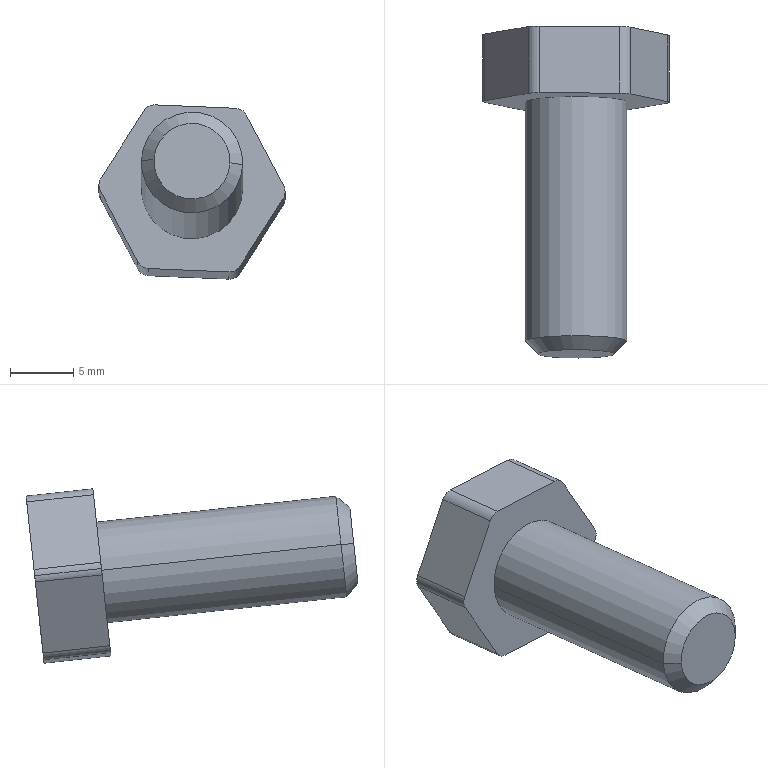Part | STEP file | Chamfer 2-4 | 1 solid | 21 faces | box 14.69 x 26.187 x 13.75 mm | volume 1768 mm3 | cylinder 10 | plane 9 | cone 2 | commonest cylinder face diameters 2 x8 8 x2
STEP:
#1=CARTESIAN_POINT('',(298.084,-1236.553,3544.637));
#2=VERTEX_POINT('',#1);
#3=CARTESIAN_POINT('',(297.929,-1236.606,3544.146));
#4=VERTEX_POINT('',#3);
#5=CARTESIAN_POINT('',(297.085,-1236.548,3544.679));
#6=DIRECTION('',(0.,0.9942,-0.1073));
#7=DIRECTION('',(0.9991,-0.004526,-0.04193));
#8=AXIS2_PLACEMENT_3D('',#5,#6,#7);
#9=CIRCLE('',#8,1.);
#10=EDGE_CURVE('',#2,#4,#9,.T.);
#11=ORIENTED_EDGE('',*,*,#10,.F.);
#12=CARTESIAN_POINT('',(298.084,-1241.822,3545.206));
#13=VERTEX_POINT('',#12);
#14=CARTESIAN_POINT('',(298.084,-1236.553,3544.637));
#15=DIRECTION('',(0.,-0.9942,0.1073));
#16=VECTOR('',#15,1000.);
#17=LINE('',#14,#16);
#18=EDGE_CURVE('',#2,#13,#17,.T.);
#19=ORIENTED_EDGE('',*,*,#18,.T.);
#20=CARTESIAN_POINT('',(297.929,-1241.875,3544.715));
#21=VERTEX_POINT('',#20);
#22=CARTESIAN_POINT('',(297.085,-1241.818,3545.248));
#23=DIRECTION('',(0.,-0.9942,0.1073));
#24=DIRECTION('',(0.9991,-0.004526,-0.04193));
#25=AXIS2_PLACEMENT_3D('',#22,#23,#24);
#26=CIRCLE('',#25,1.);
#27=EDGE_CURVE('',#21,#13,#26,.T.);
#28=ORIENTED_EDGE('',*,*,#27,.F.);
#29=CARTESIAN_POINT('',(297.929,-1236.606,3544.146));
#30=DIRECTION('',(0.,-0.9942,0.1073));
#31=VECTOR('',#30,1000.);
#32=LINE('',#29,#31);
#33=EDGE_CURVE('',#4,#21,#32,.T.);
#34=ORIENTED_EDGE('',*,*,#33,.F.);
#35=EDGE_LOOP('',(#11,#19,#28,#34));
#36=FACE_OUTER_BOUND('',#35,.T.);
#37=CARTESIAN_POINT('',(297.085,-1236.548,3544.679));
#38=DIRECTION('',(0.,-0.9942,0.1073));
#39=DIRECTION('',(0.9991,-0.004526,-0.04193));
#40=AXIS2_PLACEMENT_3D('',#37,#38,#39);
#41=CYLINDRICAL_SURFACE('',#40,1.);
#42=ADVANCED_FACE('',(#36),#41,.T.);
#43=CARTESIAN_POINT('',(287.742,-1261.66,3547.787));
#44=VERTEX_POINT('',#43);
#45=CARTESIAN_POINT('',(293.737,-1261.687,3547.536));
#46=VERTEX_POINT('',#45);
#47=CARTESIAN_POINT('',(290.74,-1261.674,3547.661));
#48=DIRECTION('',(0.,-0.9942,0.1073));
#49=DIRECTION('',(0.9991,-0.004526,-0.04193));
#50=AXIS2_PLACEMENT_3D('',#47,#48,#49);
#51=CIRCLE('',#50,3.);
#52=EDGE_CURVE('',#44,#46,#51,.T.);
#53=ORIENTED_EDGE('',*,*,#52,.F.);
#54=CARTESIAN_POINT('',(286.743,-1260.661,3547.722));
#55=VERTEX_POINT('',#54);
#56=CARTESIAN_POINT('',(286.743,-1260.661,3547.722));
#57=DIRECTION('',(-0.7065,0.7062,-0.04626));
#58=VECTOR('',#57,1000.);
#59=LINE('',#56,#58);
#60=EDGE_CURVE('',#44,#55,#59,.T.);
#61=ORIENTED_EDGE('',*,*,#60,.T.);
#62=CARTESIAN_POINT('',(294.736,-1260.697,3547.386));
#63=VERTEX_POINT('',#62);
#64=CARTESIAN_POINT('',(290.74,-1260.679,3547.554));
#65=DIRECTION('',(0.,0.9942,-0.1073));
#66=DIRECTION('',(0.9991,-0.004526,-0.04193));
#67=AXIS2_PLACEMENT_3D('',#64,#65,#66);
#68=CIRCLE('',#67,4.);
#69=EDGE_CURVE('',#63,#55,#68,.T.);
#70=ORIENTED_EDGE('',*,*,#69,.F.);
#71=CARTESIAN_POINT('',(294.736,-1260.697,3547.386));
#72=DIRECTION('',(0.7065,0.6998,-0.1055));
#73=VECTOR('',#72,1000.);
#74=LINE('',#71,#73);
#75=EDGE_CURVE('',#46,#63,#74,.T.);
#76=ORIENTED_EDGE('',*,*,#75,.F.);
#77=EDGE_LOOP('',(#53,#61,#70,#76));
#78=FACE_OUTER_BOUND('',#77,.T.);
#79=CARTESIAN_POINT('',(290.74,-1260.679,3547.554));
#80=DIRECTION('',(0.,0.9942,-0.1073));
#81=DIRECTION('',(-0.9991,0.004526,0.04193));
#82=AXIS2_PLACEMENT_3D('',#79,#80,#81);
#83=CONICAL_SURFACE('',#82,4.,0.7854);
#84=ADVANCED_FACE('',(#78),#83,.T.);
#85=ORIENTED_EDGE('',*,*,#69,.T.);
#86=CARTESIAN_POINT('',(286.743,-1241.771,3545.682));
#87=VERTEX_POINT('',#86);
#88=CARTESIAN_POINT('',(286.743,-1261.655,3547.829));
#89=DIRECTION('',(0.,0.9942,-0.1073));
#90=VECTOR('',#89,1000.);
#91=LINE('',#88,#90);
#92=EDGE_CURVE('',#55,#87,#91,.T.);
#93=ORIENTED_EDGE('',*,*,#92,.T.);
#94=CARTESIAN_POINT('',(294.736,-1241.807,3545.347));
#95=VERTEX_POINT('',#94);
#96=CARTESIAN_POINT('',(290.74,-1241.789,3545.515));
#97=DIRECTION('',(0.,0.9942,-0.1073));
#98=DIRECTION('',(0.9991,-0.004526,-0.04193));
#99=AXIS2_PLACEMENT_3D('',#96,#97,#98);
#100=CIRCLE('',#99,4.);
#101=EDGE_CURVE('',#95,#87,#100,.T.);
#102=ORIENTED_EDGE('',*,*,#101,.F.);
#103=CARTESIAN_POINT('',(294.736,-1261.692,3547.494));
#104=DIRECTION('',(0.,0.9942,-0.1073));
#105=VECTOR('',#104,1000.);
#106=LINE('',#103,#105);
#107=EDGE_CURVE('',#63,#95,#106,.T.);
#108=ORIENTED_EDGE('',*,*,#107,.F.);
#109=EDGE_LOOP('',(#85,#93,#102,#108));
#110=FACE_OUTER_BOUND('',#109,.T.);
#111=CARTESIAN_POINT('',(290.74,-1261.674,3547.661));
#112=DIRECTION('',(0.,0.9942,-0.1073));
#113=DIRECTION('',(-0.9991,0.004526,0.04193));
#114=AXIS2_PLACEMENT_3D('',#111,#112,#113);
#115=CYLINDRICAL_SURFACE('',#114,4.);
#116=ADVANCED_FACE('',(#110),#115,.T.);
#117=CARTESIAN_POINT('',(283.395,-1236.486,3545.254));
#118=VERTEX_POINT('',#117);
#119=CARTESIAN_POINT('',(283.55,-1236.433,3545.745));
#120=VERTEX_POINT('',#119);
#121=CARTESIAN_POINT('',(284.394,-1236.491,3545.212));
#122=DIRECTION('',(0.,0.9942,-0.1073));
#123=DIRECTION('',(0.9991,-0.004526,-0.04193));
#124=AXIS2_PLACEMENT_3D('',#121,#122,#123);
#125=CIRCLE('',#124,1.);
#126=EDGE_CURVE('',#118,#120,#125,.T.);
#127=ORIENTED_EDGE('',*,*,#126,.F.);
#128=CARTESIAN_POINT('',(283.395,-1241.756,3545.823));
#129=VERTEX_POINT('',#128);
#130=CARTESIAN_POINT('',(283.395,-1236.486,3545.254));
#131=DIRECTION('',(0.,-0.9942,0.1073));
#132=VECTOR('',#131,1000.);
#133=LINE('',#130,#132);
#134=EDGE_CURVE('',#118,#129,#133,.T.);
#135=ORIENTED_EDGE('',*,*,#134,.T.);
#136=CARTESIAN_POINT('',(283.55,-1241.703,3546.314));
#137=VERTEX_POINT('',#136);
#138=CARTESIAN_POINT('',(284.394,-1241.76,3545.781));
#139=DIRECTION('',(0.,-0.9942,0.1073));
#140=DIRECTION('',(0.9991,-0.004526,-0.04193));
#141=AXIS2_PLACEMENT_3D('',#138,#139,#140);
#142=CIRCLE('',#141,1.);
#143=EDGE_CURVE('',#137,#129,#142,.T.);
#144=ORIENTED_EDGE('',*,*,#143,.F.);
#145=CARTESIAN_POINT('',(283.55,-1236.433,3545.745));
#146=DIRECTION('',(0.,-0.9942,0.1073));
#147=VECTOR('',#146,1000.);
#148=LINE('',#145,#147);
#149=EDGE_CURVE('',#120,#137,#148,.T.);
#150=ORIENTED_EDGE('',*,*,#149,.F.);
#151=EDGE_LOOP('',(#127,#135,#144,#150));
#152=FACE_OUTER_BOUND('',#151,.T.);
#153=CARTESIAN_POINT('',(284.394,-1236.491,3545.212));
#154=DIRECTION('',(0.,-0.9942,0.1073));
#155=DIRECTION('',(0.9991,-0.004526,-0.04193));
#156=AXIS2_PLACEMENT_3D('',#153,#154,#155);
#157=CYLINDRICAL_SURFACE('',#156,1.);
#158=ADVANCED_FACE('',(#152),#157,.T.);
#159=CARTESIAN_POINT('',(295.03,-1235.895,3550.736));
#160=VERTEX_POINT('',#159);
#161=CARTESIAN_POINT('',(297.971,-1236.499,3545.14));
#162=VERTEX_POINT('',#161);
#163=CARTESIAN_POINT('',(294.763,-1235.84,3551.245));
#164=DIRECTION('',(0.463,-0.09514,-0.8812));
#165=VECTOR('',#164,1000.);
#166=LINE('',#163,#165);
#167=EDGE_CURVE('',#160,#162,#166,.T.);
#168=ORIENTED_EDGE('',*,*,#167,.F.);
#169=CARTESIAN_POINT('',(295.03,-1241.164,3551.305));
#170=VERTEX_POINT('',#169);
#171=CARTESIAN_POINT('',(295.03,-1235.895,3550.736));
#172=DIRECTION('',(0.,-0.9942,0.1073));
#173=VECTOR('',#172,1000.);
#174=LINE('',#171,#173);
#175=EDGE_CURVE('',#160,#170,#174,.T.);
#176=ORIENTED_EDGE('',*,*,#175,.T.);
#177=CARTESIAN_POINT('',(297.971,-1241.768,3545.709));
#178=VERTEX_POINT('',#177);
#179=CARTESIAN_POINT('',(294.763,-1241.109,3551.814));
#180=DIRECTION('',(0.463,-0.09514,-0.8812));
#181=VECTOR('',#180,1000.);
#182=LINE('',#179,#181);
#183=EDGE_CURVE('',#170,#178,#182,.T.);
#184=ORIENTED_EDGE('',*,*,#183,.T.);
#185=CARTESIAN_POINT('',(297.971,-1236.499,3545.14));
#186=DIRECTION('',(0.,0.9942,-0.1073));
#187=VECTOR('',#186,1000.);
#188=LINE('',#185,#187);
#189=EDGE_CURVE('',#178,#162,#188,.T.);
#190=ORIENTED_EDGE('',*,*,#189,.T.);
#191=EDGE_LOOP('',(#168,#176,#184,#190));
#192=FACE_OUTER_BOUND('',#191,.T.);
#193=CARTESIAN_POINT('',(294.763,-1235.84,3551.245));
#194=DIRECTION('',(-0.8863,-0.0497,-0.4604));
#195=DIRECTION('',(0.463,-0.09514,-0.8812));
#196=AXIS2_PLACEMENT_3D('',#193,#194,#195);
#197=PLANE('',#196);
#198=ADVANCED_FACE('',(#192),#197,.F.);
#199=CARTESIAN_POINT('',(294.524,-1242.451,3539.385));
#200=VERTEX_POINT('',#199);
#201=CARTESIAN_POINT('',(298.238,-1241.823,3545.2));
#202=DIRECTION('',(-0.5361,-0.09061,-0.8393));
#203=VECTOR('',#202,1000.);
#204=LINE('',#201,#203);
#205=EDGE_CURVE('',#21,#200,#204,.T.);
#206=ORIENTED_EDGE('',*,*,#205,.T.);
#207=CARTESIAN_POINT('',(294.524,-1237.181,3538.816));
#208=VERTEX_POINT('',#207);
#209=CARTESIAN_POINT('',(294.524,-1237.181,3538.816));
#210=DIRECTION('',(0.,0.9942,-0.1073));
#211=VECTOR('',#210,1000.);
#212=LINE('',#209,#211);
#213=EDGE_CURVE('',#200,#208,#212,.T.);
#214=ORIENTED_EDGE('',*,*,#213,.T.);
#215=CARTESIAN_POINT('',(298.238,-1236.554,3544.631));
#216=DIRECTION('',(-0.5361,-0.09061,-0.8393));
#217=VECTOR('',#216,1000.);
#218=LINE('',#215,#217);
#219=EDGE_CURVE('',#4,#208,#218,.T.);
#220=ORIENTED_EDGE('',*,*,#219,.F.);
#221=ORIENTED_EDGE('',*,*,#33,.T.);
#222=EDGE_LOOP('',(#206,#214,#220,#221));
#223=FACE_OUTER_BOUND('',#222,.T.);
#224=CARTESIAN_POINT('',(298.238,-1236.554,3544.631));
#225=DIRECTION('',(-0.8442,0.05754,0.533));
#226=DIRECTION('',(-0.5361,-0.09061,-0.8393));
#227=AXIS2_PLACEMENT_3D('',#224,#225,#226);
#228=PLANE('',#227);
#229=ADVANCED_FACE('',(#223),#228,.F.);
#230=CARTESIAN_POINT('',(293.638,-1237.231,3538.356));
#231=VERTEX_POINT('',#230);
#232=CARTESIAN_POINT('',(287.293,-1237.202,3538.622));
#233=VERTEX_POINT('',#232);
#234=CARTESIAN_POINT('',(294.215,-1237.234,3538.332));
#235=DIRECTION('',(-0.9991,0.004526,0.04193));
#236=VECTOR('',#235,1000.);
#237=LINE('',#234,#236);
#238=EDGE_CURVE('',#231,#233,#237,.T.);
#239=ORIENTED_EDGE('',*,*,#238,.F.);
#240=CARTESIAN_POINT('',(293.638,-1242.501,3538.925));
#241=VERTEX_POINT('',#240);
#242=CARTESIAN_POINT('',(293.638,-1237.231,3538.356));
#243=DIRECTION('',(0.,-0.9942,0.1073));
#244=VECTOR('',#243,1000.);
#245=LINE('',#242,#244);
#246=EDGE_CURVE('',#231,#241,#245,.T.);
#247=ORIENTED_EDGE('',*,*,#246,.T.);
#248=CARTESIAN_POINT('',(287.293,-1242.472,3539.191));
#249=VERTEX_POINT('',#248);
#250=CARTESIAN_POINT('',(294.215,-1242.503,3538.901));
#251=DIRECTION('',(-0.9991,0.004526,0.04193));
#252=VECTOR('',#251,1000.);
#253=LINE('',#250,#252);
#254=EDGE_CURVE('',#241,#249,#253,.T.);
#255=ORIENTED_EDGE('',*,*,#254,.T.);
#256=CARTESIAN_POINT('',(287.293,-1237.202,3538.622));
#257=DIRECTION('',(0.,0.9942,-0.1073));
#258=VECTOR('',#257,1000.);
#259=LINE('',#256,#258);
#260=EDGE_CURVE('',#249,#233,#259,.T.);
#261=ORIENTED_EDGE('',*,*,#260,.T.);
#262=EDGE_LOOP('',(#239,#247,#255,#261));
#263=FACE_OUTER_BOUND('',#262,.T.);
#264=CARTESIAN_POINT('',(294.215,-1237.234,3538.332));
#265=DIRECTION('',(0.04217,0.1072,0.9933));
#266=DIRECTION('',(0.,0.9942,-0.1073));
#267=AXIS2_PLACEMENT_3D('',#264,#265,#266);
#268=PLANE('',#267);
#269=ADVANCED_FACE('',(#263),#268,.F.);
#270=CARTESIAN_POINT('',(286.449,-1237.145,3539.155));
#271=VERTEX_POINT('',#270);
#272=CARTESIAN_POINT('',(283.508,-1236.541,3544.752));
#273=VERTEX_POINT('',#272);
#274=CARTESIAN_POINT('',(286.716,-1237.2,3538.646));
#275=DIRECTION('',(-0.463,0.09514,0.8812));
#276=VECTOR('',#275,1000.);
#277=LINE('',#274,#276);
#278=EDGE_CURVE('',#271,#273,#277,.T.);
#279=ORIENTED_EDGE('',*,*,#278,.F.);
#280=CARTESIAN_POINT('',(286.449,-1242.414,3539.724));
#281=VERTEX_POINT('',#280);
#282=CARTESIAN_POINT('',(286.449,-1237.145,3539.155));
#283=DIRECTION('',(0.,-0.9942,0.1073));
#284=VECTOR('',#283,1000.);
#285=LINE('',#282,#284);
#286=EDGE_CURVE('',#271,#281,#285,.T.);
#287=ORIENTED_EDGE('',*,*,#286,.T.);
#288=CARTESIAN_POINT('',(283.508,-1241.81,3545.32));
#289=VERTEX_POINT('',#288);
#290=CARTESIAN_POINT('',(286.716,-1242.469,3539.215));
#291=DIRECTION('',(-0.463,0.09514,0.8812));
#292=VECTOR('',#291,1000.);
#293=LINE('',#290,#292);
#294=EDGE_CURVE('',#281,#289,#293,.T.);
#295=ORIENTED_EDGE('',*,*,#294,.T.);
#296=CARTESIAN_POINT('',(283.508,-1236.541,3544.752));
#297=DIRECTION('',(0.,0.9942,-0.1073));
#298=VECTOR('',#297,1000.);
#299=LINE('',#296,#298);
#300=EDGE_CURVE('',#289,#273,#299,.T.);
#301=ORIENTED_EDGE('',*,*,#300,.T.);
#302=EDGE_LOOP('',(#279,#287,#295,#301));
#303=FACE_OUTER_BOUND('',#302,.T.);
#304=CARTESIAN_POINT('',(286.716,-1237.2,3538.646));
#305=DIRECTION('',(0.8863,0.0497,0.4604));
#306=DIRECTION('',(-0.463,0.09514,0.8812));
#307=AXIS2_PLACEMENT_3D('',#304,#305,#306);
#308=PLANE('',#307);
#309=ADVANCED_FACE('',(#303),#308,.F.);
#310=CARTESIAN_POINT('',(286.955,-1235.858,3551.075));
#311=VERTEX_POINT('',#310);
#312=CARTESIAN_POINT('',(283.241,-1236.486,3545.26));
#313=DIRECTION('',(0.5361,0.09061,0.8393));
#314=VECTOR('',#313,1000.);
#315=LINE('',#312,#314);
#316=EDGE_CURVE('',#120,#311,#315,.T.);
#317=ORIENTED_EDGE('',*,*,#316,.F.);
#318=ORIENTED_EDGE('',*,*,#149,.T.);
#319=CARTESIAN_POINT('',(286.955,-1241.127,3551.644));
#320=VERTEX_POINT('',#319);
#321=CARTESIAN_POINT('',(283.241,-1241.755,3545.829));
#322=DIRECTION('',(0.5361,0.09061,0.8393));
#323=VECTOR('',#322,1000.);
#324=LINE('',#321,#323);
#325=EDGE_CURVE('',#137,#320,#324,.T.);
#326=ORIENTED_EDGE('',*,*,#325,.T.);
#327=CARTESIAN_POINT('',(286.955,-1235.858,3551.075));
#328=DIRECTION('',(0.,0.9942,-0.1073));
#329=VECTOR('',#328,1000.);
#330=LINE('',#327,#329);
#331=EDGE_CURVE('',#320,#311,#330,.T.);
#332=ORIENTED_EDGE('',*,*,#331,.T.);
#333=EDGE_LOOP('',(#317,#318,#326,#332));
#334=FACE_OUTER_BOUND('',#333,.T.);
#335=CARTESIAN_POINT('',(283.241,-1236.486,3545.26));
#336=DIRECTION('',(0.8442,-0.05754,-0.533));
#337=DIRECTION('',(0.5361,0.09061,0.8393));
#338=AXIS2_PLACEMENT_3D('',#335,#336,#337);
#339=PLANE('',#338);
#340=ADVANCED_FACE('',(#334),#339,.F.);
#341=CARTESIAN_POINT('',(287.841,-1235.808,3551.535));
#342=VERTEX_POINT('',#341);
#343=CARTESIAN_POINT('',(294.186,-1235.837,3551.269));
#344=VERTEX_POINT('',#343);
#345=CARTESIAN_POINT('',(287.264,-1235.806,3551.56));
#346=DIRECTION('',(0.9991,-0.004526,-0.04193));
#347=VECTOR('',#346,1000.);
#348=LINE('',#345,#347);
#349=EDGE_CURVE('',#342,#344,#348,.T.);
#350=ORIENTED_EDGE('',*,*,#349,.F.);
#351=CARTESIAN_POINT('',(287.841,-1241.078,3552.104));
#352=VERTEX_POINT('',#351);
#353=CARTESIAN_POINT('',(287.841,-1235.808,3551.535));
#354=DIRECTION('',(0.,-0.9942,0.1073));
#355=VECTOR('',#354,1000.);
#356=LINE('',#353,#355);
#357=EDGE_CURVE('',#342,#352,#356,.T.);
#358=ORIENTED_EDGE('',*,*,#357,.T.);
#359=CARTESIAN_POINT('',(294.186,-1241.106,3551.838));
#360=VERTEX_POINT('',#359);
#361=CARTESIAN_POINT('',(287.264,-1241.075,3552.129));
#362=DIRECTION('',(0.9991,-0.004526,-0.04193));
#363=VECTOR('',#362,1000.);
#364=LINE('',#361,#363);
#365=EDGE_CURVE('',#352,#360,#364,.T.);
#366=ORIENTED_EDGE('',*,*,#365,.T.);
#367=CARTESIAN_POINT('',(294.186,-1235.837,3551.269));
#368=DIRECTION('',(0.,0.9942,-0.1073));
#369=VECTOR('',#368,1000.);
#370=LINE('',#367,#369);
#371=EDGE_CURVE('',#360,#344,#370,.T.);
#372=ORIENTED_EDGE('',*,*,#371,.T.);
#373=EDGE_LOOP('',(#350,#358,#366,#372));
#374=FACE_OUTER_BOUND('',#373,.T.);
#375=CARTESIAN_POINT('',(287.264,-1235.806,3551.56));
#376=DIRECTION('',(-0.04217,-0.1072,-0.9933));
#377=DIRECTION('',(0.9991,-0.004526,-0.04193));
#378=AXIS2_PLACEMENT_3D('',#375,#376,#377);
#379=PLANE('',#378);
#380=ADVANCED_FACE('',(#374),#379,.F.);
#381=ORIENTED_EDGE('',*,*,#219,.T.);
#382=CARTESIAN_POINT('',(293.68,-1237.124,3539.349));
#383=DIRECTION('',(0.,0.9942,-0.1073));
#384=DIRECTION('',(0.9991,-0.004526,-0.04193));
#385=AXIS2_PLACEMENT_3D('',#382,#383,#384);
#386=CIRCLE('',#385,1.);
#387=EDGE_CURVE('',#208,#231,#386,.T.);
#388=ORIENTED_EDGE('',*,*,#387,.T.);
#389=ORIENTED_EDGE('',*,*,#238,.T.);
#390=CARTESIAN_POINT('',(287.335,-1237.095,3539.615));
#391=DIRECTION('',(0.,0.9942,-0.1073));
#392=DIRECTION('',(0.9991,-0.004526,-0.04193));
#393=AXIS2_PLACEMENT_3D('',#390,#391,#392);
#394=CIRCLE('',#393,1.);
#395=EDGE_CURVE('',#233,#271,#394,.T.);
#396=ORIENTED_EDGE('',*,*,#395,.T.);
#397=ORIENTED_EDGE('',*,*,#278,.T.);
#398=CARTESIAN_POINT('',(284.394,-1236.491,3545.212));
#399=DIRECTION('',(0.,0.9942,-0.1073));
#400=DIRECTION('',(0.9991,-0.004526,-0.04193));
#401=AXIS2_PLACEMENT_3D('',#398,#399,#400);
#402=CIRCLE('',#401,1.);
#403=EDGE_CURVE('',#273,#118,#402,.T.);
#404=ORIENTED_EDGE('',*,*,#403,.T.);
#405=ORIENTED_EDGE('',*,*,#126,.T.);
#406=ORIENTED_EDGE('',*,*,#316,.T.);
#407=CARTESIAN_POINT('',(287.799,-1235.915,3550.542));
#408=DIRECTION('',(0.,0.9942,-0.1073));
#409=DIRECTION('',(0.9991,-0.004526,-0.04193));
#410=AXIS2_PLACEMENT_3D('',#407,#408,#409);
#411=CIRCLE('',#410,1.);
#412=EDGE_CURVE('',#311,#342,#411,.T.);
#413=ORIENTED_EDGE('',*,*,#412,.T.);
#414=ORIENTED_EDGE('',*,*,#349,.T.);
#415=CARTESIAN_POINT('',(294.144,-1235.944,3550.276));
#416=DIRECTION('',(0.,0.9942,-0.1073));
#417=DIRECTION('',(0.9991,-0.004526,-0.04193));
#418=AXIS2_PLACEMENT_3D('',#415,#416,#417);
#419=CIRCLE('',#418,1.);
#420=EDGE_CURVE('',#344,#160,#419,.T.);
#421=ORIENTED_EDGE('',*,*,#420,.T.);
#422=ORIENTED_EDGE('',*,*,#167,.T.);
#423=CARTESIAN_POINT('',(297.085,-1236.548,3544.679));
#424=DIRECTION('',(0.,0.9942,-0.1073));
#425=DIRECTION('',(0.9991,-0.004526,-0.04193));
#426=AXIS2_PLACEMENT_3D('',#423,#424,#425);
#427=CIRCLE('',#426,1.);
#428=EDGE_CURVE('',#162,#2,#427,.T.);
#429=ORIENTED_EDGE('',*,*,#428,.T.);
#430=ORIENTED_EDGE('',*,*,#10,.T.);
#431=EDGE_LOOP('',(#381,#388,#389,#396,#397,#404,#405,#406,#413,#414,#421,#422,#429,#430));
#432=FACE_OUTER_BOUND('',#431,.T.);
#433=CARTESIAN_POINT('',(293.975,-1236.534,3544.81));
#434=DIRECTION('',(0.,0.9942,-0.1073));
#435=DIRECTION('',(-0.9991,0.004526,0.04193));
#436=AXIS2_PLACEMENT_3D('',#433,#434,#435);
#437=PLANE('',#436);
#438=ADVANCED_FACE('',(#432),#437,.T.);
#439=ORIENTED_EDGE('',*,*,#101,.T.);
#440=CARTESIAN_POINT('',(290.74,-1241.789,3545.515));
#441=DIRECTION('',(0.,0.9942,-0.1073));
#442=DIRECTION('',(0.9991,-0.004526,-0.04193));
#443=AXIS2_PLACEMENT_3D('',#440,#441,#442);
#444=CIRCLE('',#443,4.);
#445=EDGE_CURVE('',#87,#95,#444,.T.);
#446=ORIENTED_EDGE('',*,*,#445,.T.);
#447=EDGE_LOOP('',(#439,#446));
#448=FACE_BOUND('',#447,.T.);
#449=ORIENTED_EDGE('',*,*,#254,.F.);
#450=CARTESIAN_POINT('',(293.68,-1242.393,3539.918));
#451=DIRECTION('',(0.,-0.9942,0.1073));
#452=DIRECTION('',(0.9991,-0.004526,-0.04193));
#453=AXIS2_PLACEMENT_3D('',#450,#451,#452);
#454=CIRCLE('',#453,1.);
#455=EDGE_CURVE('',#241,#200,#454,.T.);
#456=ORIENTED_EDGE('',*,*,#455,.T.);
#457=ORIENTED_EDGE('',*,*,#205,.F.);
#458=ORIENTED_EDGE('',*,*,#27,.T.);
#459=CARTESIAN_POINT('',(297.085,-1241.818,3545.248));
#460=DIRECTION('',(0.,-0.9942,0.1073));
#461=DIRECTION('',(0.9991,-0.004526,-0.04193));
#462=AXIS2_PLACEMENT_3D('',#459,#460,#461);
#463=CIRCLE('',#462,1.);
#464=EDGE_CURVE('',#13,#178,#463,.T.);
#465=ORIENTED_EDGE('',*,*,#464,.T.);
#466=ORIENTED_EDGE('',*,*,#183,.F.);
#467=CARTESIAN_POINT('',(294.144,-1241.214,3550.845));
#468=DIRECTION('',(0.,-0.9942,0.1073));
#469=DIRECTION('',(0.9991,-0.004526,-0.04193));
#470=AXIS2_PLACEMENT_3D('',#467,#468,#469);
#471=CIRCLE('',#470,1.);
#472=EDGE_CURVE('',#170,#360,#471,.T.);
#473=ORIENTED_EDGE('',*,*,#472,.T.);
#474=ORIENTED_EDGE('',*,*,#365,.F.);
#475=CARTESIAN_POINT('',(287.799,-1241.185,3551.111));
#476=DIRECTION('',(0.,-0.9942,0.1073));
#477=DIRECTION('',(0.9991,-0.004526,-0.04193));
#478=AXIS2_PLACEMENT_3D('',#475,#476,#477);
#479=CIRCLE('',#478,1.);
#480=EDGE_CURVE('',#352,#320,#479,.T.);
#481=ORIENTED_EDGE('',*,*,#480,.T.);
#482=ORIENTED_EDGE('',*,*,#325,.F.);
#483=ORIENTED_EDGE('',*,*,#143,.T.);
#484=CARTESIAN_POINT('',(284.394,-1241.76,3545.781));
#485=DIRECTION('',(0.,-0.9942,0.1073));
#486=DIRECTION('',(0.9991,-0.004526,-0.04193));
#487=AXIS2_PLACEMENT_3D('',#484,#485,#486);
#488=CIRCLE('',#487,1.);
#489=EDGE_CURVE('',#129,#289,#488,.T.);
#490=ORIENTED_EDGE('',*,*,#489,.T.);
#491=ORIENTED_EDGE('',*,*,#294,.F.);
#492=CARTESIAN_POINT('',(287.335,-1242.365,3540.184));
#493=DIRECTION('',(0.,-0.9942,0.1073));
#494=DIRECTION('',(0.9991,-0.004526,-0.04193));
#495=AXIS2_PLACEMENT_3D('',#492,#493,#494);
#496=CIRCLE('',#495,1.);
#497=EDGE_CURVE('',#281,#249,#496,.T.);
#498=ORIENTED_EDGE('',*,*,#497,.T.);
#499=EDGE_LOOP('',(#449,#456,#457,#458,#465,#466,#473,#474,#481,#482,#483,#490,#491,#498));
#500=FACE_OUTER_BOUND('',#499,.T.);
#501=CARTESIAN_POINT('',(293.975,-1241.804,3545.379));
#502=DIRECTION('',(0.,0.9942,-0.1073));
#503=DIRECTION('',(-0.9991,0.004526,0.04193));
#504=AXIS2_PLACEMENT_3D('',#501,#502,#503);
#505=PLANE('',#504);
#506=ADVANCED_FACE('',(#448,#500),#505,.F.);
#507=ORIENTED_EDGE('',*,*,#387,.F.);
#508=ORIENTED_EDGE('',*,*,#213,.F.);
#509=ORIENTED_EDGE('',*,*,#455,.F.);
#510=ORIENTED_EDGE('',*,*,#246,.F.);
#511=EDGE_LOOP('',(#507,#508,#509,#510));
#512=FACE_OUTER_BOUND('',#511,.T.);
#513=CARTESIAN_POINT('',(293.68,-1237.124,3539.349));
#514=DIRECTION('',(0.,-0.9942,0.1073));
#515=DIRECTION('',(0.9991,-0.004526,-0.04193));
#516=AXIS2_PLACEMENT_3D('',#513,#514,#515);
#517=CYLINDRICAL_SURFACE('',#516,1.);
#518=ADVANCED_FACE('',(#512),#517,.T.);
#519=ORIENTED_EDGE('',*,*,#395,.F.);
#520=ORIENTED_EDGE('',*,*,#260,.F.);
#521=ORIENTED_EDGE('',*,*,#497,.F.);
#522=ORIENTED_EDGE('',*,*,#286,.F.);
#523=EDGE_LOOP('',(#519,#520,#521,#522));
#524=FACE_OUTER_BOUND('',#523,.T.);
#525=CARTESIAN_POINT('',(287.335,-1237.095,3539.615));
#526=DIRECTION('',(0.,-0.9942,0.1073));
#527=DIRECTION('',(0.9991,-0.004526,-0.04193));
#528=AXIS2_PLACEMENT_3D('',#525,#526,#527);
#529=CYLINDRICAL_SURFACE('',#528,1.);
#530=ADVANCED_FACE('',(#524),#529,.T.);
#531=ORIENTED_EDGE('',*,*,#134,.F.);
#532=ORIENTED_EDGE('',*,*,#403,.F.);
#533=ORIENTED_EDGE('',*,*,#300,.F.);
#534=ORIENTED_EDGE('',*,*,#489,.F.);
#535=EDGE_LOOP('',(#531,#532,#533,#534));
#536=FACE_OUTER_BOUND('',#535,.T.);
#537=CARTESIAN_POINT('',(284.394,-1236.491,3545.212));
#538=DIRECTION('',(0.,-0.9942,0.1073));
#539=DIRECTION('',(0.9991,-0.004526,-0.04193));
#540=AXIS2_PLACEMENT_3D('',#537,#538,#539);
#541=CYLINDRICAL_SURFACE('',#540,1.);
#542=ADVANCED_FACE('',(#536),#541,.T.);
#543=ORIENTED_EDGE('',*,*,#412,.F.);
#544=ORIENTED_EDGE('',*,*,#331,.F.);
#545=ORIENTED_EDGE('',*,*,#480,.F.);
#546=ORIENTED_EDGE('',*,*,#357,.F.);
#547=EDGE_LOOP('',(#543,#544,#545,#546));
#548=FACE_OUTER_BOUND('',#547,.T.);
#549=CARTESIAN_POINT('',(287.799,-1235.915,3550.542));
#550=DIRECTION('',(0.,-0.9942,0.1073));
#551=DIRECTION('',(0.9991,-0.004526,-0.04193));
#552=AXIS2_PLACEMENT_3D('',#549,#550,#551);
#553=CYLINDRICAL_SURFACE('',#552,1.);
#554=ADVANCED_FACE('',(#548),#553,.T.);
#555=ORIENTED_EDGE('',*,*,#420,.F.);
#556=ORIENTED_EDGE('',*,*,#371,.F.);
#557=ORIENTED_EDGE('',*,*,#472,.F.);
#558=ORIENTED_EDGE('',*,*,#175,.F.);
#559=EDGE_LOOP('',(#555,#556,#557,#558));
#560=FACE_OUTER_BOUND('',#559,.T.);
#561=CARTESIAN_POINT('',(294.144,-1235.944,3550.276));
#562=DIRECTION('',(0.,-0.9942,0.1073));
#563=DIRECTION('',(0.9991,-0.004526,-0.04193));
#564=AXIS2_PLACEMENT_3D('',#561,#562,#563);
#565=CYLINDRICAL_SURFACE('',#564,1.);
#566=ADVANCED_FACE('',(#560),#565,.T.);
#567=ORIENTED_EDGE('',*,*,#18,.F.);
#568=ORIENTED_EDGE('',*,*,#428,.F.);
#569=ORIENTED_EDGE('',*,*,#189,.F.);
#570=ORIENTED_EDGE('',*,*,#464,.F.);
#571=EDGE_LOOP('',(#567,#568,#569,#570));
#572=FACE_OUTER_BOUND('',#571,.T.);
#573=CARTESIAN_POINT('',(297.085,-1236.548,3544.679));
#574=DIRECTION('',(0.,-0.9942,0.1073));
#575=DIRECTION('',(0.9991,-0.004526,-0.04193));
#576=AXIS2_PLACEMENT_3D('',#573,#574,#575);
#577=CYLINDRICAL_SURFACE('',#576,1.);
#578=ADVANCED_FACE('',(#572),#577,.T.);
#579=ORIENTED_EDGE('',*,*,#92,.F.);
#580=CARTESIAN_POINT('',(290.74,-1260.679,3547.554));
#581=DIRECTION('',(0.,0.9942,-0.1073));
#582=DIRECTION('',(0.9991,-0.004526,-0.04193));
#583=AXIS2_PLACEMENT_3D('',#580,#581,#582);
#584=CIRCLE('',#583,4.);
#585=EDGE_CURVE('',#55,#63,#584,.T.);
#586=ORIENTED_EDGE('',*,*,#585,.T.);
#587=ORIENTED_EDGE('',*,*,#107,.T.);
#588=ORIENTED_EDGE('',*,*,#445,.F.);
#589=EDGE_LOOP('',(#579,#586,#587,#588));
#590=FACE_OUTER_BOUND('',#589,.T.);
#591=CARTESIAN_POINT('',(290.74,-1261.674,3547.661));
#592=DIRECTION('',(0.,0.9942,-0.1073));
#593=DIRECTION('',(-0.9991,0.004526,0.04193));
#594=AXIS2_PLACEMENT_3D('',#591,#592,#593);
#595=CYLINDRICAL_SURFACE('',#594,4.);
#596=ADVANCED_FACE('',(#590),#595,.T.);
#597=CARTESIAN_POINT('',(290.74,-1261.674,3547.661));
#598=DIRECTION('',(0.,-0.9942,0.1073));
#599=DIRECTION('',(0.9991,-0.004526,-0.04193));
#600=AXIS2_PLACEMENT_3D('',#597,#598,#599);
#601=CIRCLE('',#600,3.);
#602=EDGE_CURVE('',#46,#44,#601,.T.);
#603=ORIENTED_EDGE('',*,*,#602,.T.);
#604=ORIENTED_EDGE('',*,*,#52,.T.);
#605=EDGE_LOOP('',(#603,#604));
#606=FACE_OUTER_BOUND('',#605,.T.);
#607=CARTESIAN_POINT('',(290.74,-1261.674,3547.661));
#608=DIRECTION('',(0.,0.9942,-0.1073));
#609=DIRECTION('',(-0.9991,0.004526,0.04193));
#610=AXIS2_PLACEMENT_3D('',#607,#608,#609);
#611=PLANE('',#610);
#612=ADVANCED_FACE('',(#606),#611,.F.);
#613=ORIENTED_EDGE('',*,*,#60,.F.);
#614=ORIENTED_EDGE('',*,*,#602,.F.);
#615=ORIENTED_EDGE('',*,*,#75,.T.);
#616=ORIENTED_EDGE('',*,*,#585,.F.);
#617=EDGE_LOOP('',(#613,#614,#615,#616));
#618=FACE_OUTER_BOUND('',#617,.T.);
#619=CARTESIAN_POINT('',(290.74,-1260.679,3547.554));
#620=DIRECTION('',(0.,0.9942,-0.1073));
#621=DIRECTION('',(-0.9991,0.004526,0.04193));
#622=AXIS2_PLACEMENT_3D('',#619,#620,#621);
#623=CONICAL_SURFACE('',#622,4.,0.7854);
#624=ADVANCED_FACE('',(#618),#623,.T.);
#625=CLOSED_SHELL('',(#42,#84,#116,#158,#198,#229,#269,#309,#340,#380,#438,#506,#518,#530,#542,#554,#566,#578,#596,#612,#624));
#626=MANIFOLD_SOLID_BREP('',#625);
#627=CARTESIAN_POINT('',(0.,0.,0.));
#628=DIRECTION('',(0.,0.,1.));
#629=DIRECTION('',(1.,0.,0.));
#630=AXIS2_PLACEMENT_3D('',#627,#628,#629);
#631=(LENGTH_UNIT()NAMED_UNIT(*)SI_UNIT(.MILLI.,.METRE.));
#632=UNCERTAINTY_MEASURE_WITH_UNIT(LENGTH_MEASURE(0.00001),#631,'','');
#633=(NAMED_UNIT(*)PLANE_ANGLE_UNIT()SI_UNIT($,.RADIAN.));
#634=(NAMED_UNIT(*)SI_UNIT($,.STERADIAN.)SOLID_ANGLE_UNIT());
#635=(GEOMETRIC_REPRESENTATION_CONTEXT(3)GLOBAL_UNCERTAINTY_ASSIGNED_CONTEXT((#632))GLOBAL_UNIT_ASSIGNED_CONTEXT((#631,#633,#634))REPRESENTATION_CONTEXT('',''));
#636=ADVANCED_BREP_SHAPE_REPRESENTATION('',(#626,#630),#635);